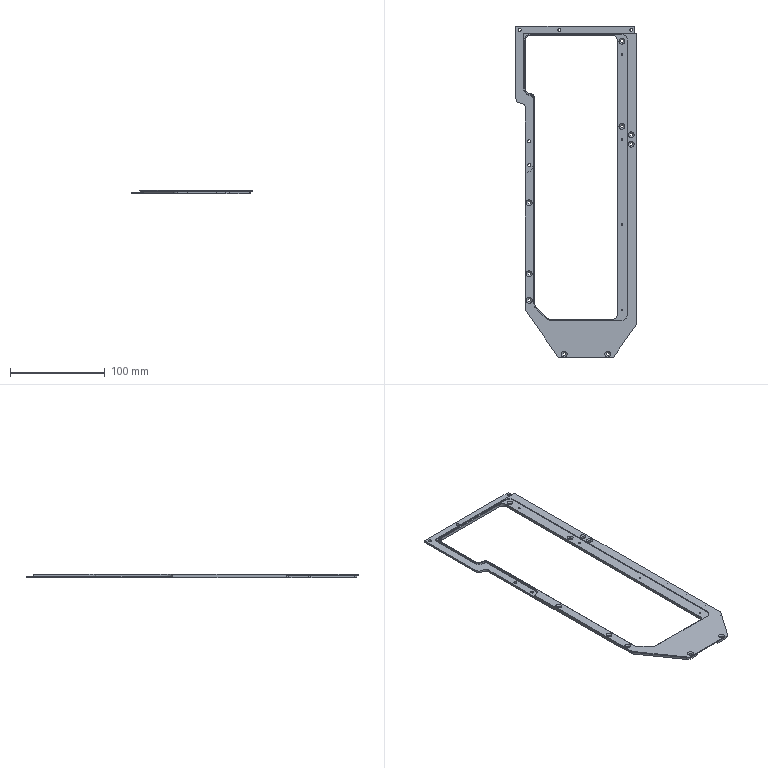NC program | NX | posted with a generic post | part box 127 x 351 x 4 mm
Whole program:
N10 G17 G21 G94 G90
(DRILLING , TOOL : CHAMFER_D8-90DEG)
N12 T01 M6
N14 G54
N16 G17 G0 G90 X-8. Y49.5 S2500 M3
N18 G43 Z20. H1
N20 G94 G81 G99 Z-2.8 F250. R3.
N22 X-83.
N24 X-111.
N26 X-168. Y12.5
N28 Y-33.5
N30 X54. Y-58.5
N32 X64.
N34 G80
N36 G0 X64. Y-58.5 Z20.
N38 M5
(PLANAR_MILL_2 , TOOL : D6-18-D6-50-3T-ROUGH)
N40 T03 M6
N42 G54
N44 G17 G0 G90 X31.2 Y59.5 S3500 M3
N46 G43 Z20. H3
N48 Z2.05
N50 G94 G1 Z-0.95 F1000.
N52 Y53.5
N54 G3 X32. Y52.7 R0.8
N56 G1 X98.935
N58 G2 X112.5 Y62.7 R14.2
N60 G1 X170.9
N62 G2 X178.2 Y55.4 R7.3
N64 G1 Y-64.6
N66 Y-70.6
N68 Z2.05
N70 G0 Z20.
N72 X27. Y59.5
N74 Z2.05
N76 G1 Z-0.95
N78 Y53.5
N80 G3 X32. Y48.5 R5.
N82 G1 X102.5
N84 G2 X112.5 Y58.5 R10.
N86 G1 X170.9
N88 G2 X174. Y55.4 R3.1
N90 G1 Y-64.6
N92 Y-70.6
N94 Z2.05
N96 G0 Z20.
N98 X31.2 Y59.5
N100 Z1.1
N102 G1 Z-1.9
N104 Y53.5
N106 G3 X32. Y52.7 R0.8
N108 G1 X98.935
N110 G2 X112.5 Y62.7 R14.2
N112 G1 X170.9
N114 G2 X178.2 Y55.4 R7.3
N116 G1 Y-64.6
N118 Y-70.6
N120 Z1.1
N122 G0 Z20.
N124 X27. Y59.5
N126 Z1.1
N128 G1 Z-1.9
N130 Y53.5
N132 G3 X32. Y48.5 R5.
N134 G1 X102.5
N136 G2 X112.5 Y58.5 R10.
N138 G1 X170.9
N140 G2 X174. Y55.4 R3.1
N142 G1 Y-64.6
N144 Y-70.6
N146 Z1.1
N148 G0 Z20.
(PLANAR_MILL_2_COPY , TOOL : D6-18-D6-50-3T-ROUGH)
N150 X90.5 Y57.5
N152 Z0.1
N154 G1 Z-1.9
N156 Y54.5
N158 G3 X92.5 Y52.5 R2.
N160 X98.5 Y58.5 R6.
N162 G2 X102.5 Y62.5 R4.
N164 G1 X175.
N166 G2 X178. Y59.5 R3.
N168 G1 Y48.5
N170 G3 X180. Y46.5 R2.
N172 G1 X183.
N174 Z0.1
N176 G0 Z20.
(PLANAR_MILL_3_COPY , TOOL : D6-18-D6-50-3T-ROUGH)
N178 X-123.5 Y-37.5
N180 Z2.1
N182 G1 Z-0.9
N184 Y-43.5
N186 Y-46.
N188 X161.5
N190 Y-43.5
N192 Y-37.5
N194 Z2.1
N196 G0 Z20.
(PLANAR_MILL_3 , TOOL : D6-18-D6-50-3T-ROUGH)
N198 X163.9 Y-48.4
N200 Z2.1
N202 G1 Z-0.9
N204 X164.
N206 Y-51.4
N208 G3 X166.9 Y-48.5 R2.9
N210 G1 Y48.5
N212 G3 X164. Y51.4 R2.9
N214 G1 X112.5
N216 G3 X109.6 Y48.5 R2.9
N218 G2 X102.5 Y41.4 R7.1
N220 G1 X-114.787
N222 G3 X-116.837 Y40.551 R2.9
N224 G1 X-128.051 Y29.337
N226 G3 X-128.9 Y27.287 R2.9
N228 G1 Y-48.5
N230 G3 X-126. Y-51.4 R2.9
N232 G1 X164.
N234 Y-48.4
N236 X163.9
N238 Z2.1
N240 G0 Z20.
N242 M5
(PLANAR_MILL_2_COPY_1 , TOOL : D6-18-D6-50-3T-FINISH)
N244 T04 M6
N246 G54
N248 G17 G0 G90 X31.1 Y59.5 S3500 M3
N250 G43 Z20. H4
N252 Z1.
N254 G94 G1 Z-2. F1000.
N256 Y53.5
N258 G3 X32. Y52.6 R0.9
N260 G1 X99.009
N262 G2 X112.5 Y62.6 R14.1
N264 G1 X170.9
N266 G2 X178.1 Y55.4 R7.2
N268 G1 Y-64.6
N270 Y-70.6
N272 Z1.
N274 G0 Z20.
N276 X26.9 Y59.5
N278 Z1.
N280 G1 Z-2.
N282 Y53.5
N284 G3 X32. Y48.4 R5.1
N286 G1 X102.5
N288 X102.565 Y48.387
N290 X102.613 Y48.435
N292 X102.6 Y48.5
N294 G2 X112.5 Y58.4 R9.9
N296 G1 X170.9
N298 G2 X173.9 Y55.4 R3.
N300 G1 Y-64.6
N302 Y-70.6
N304 Z1.
N306 G0 Z20.
(PLANAR_MILL_2_COPY_COPY , TOOL : D6-18-D6-50-3T-FINISH)
N308 X90.5 Y57.5
N310 Z0.
N312 G1 Z-2.
N314 Y54.5
N316 G3 X92.5 Y52.5 R2.
N318 X98.5 Y58.5 R6.
N320 G2 X102.5 Y62.5 R4.
N322 G1 X175.
N324 G2 X178. Y59.5 R3.
N326 G1 Y48.5
N328 G3 X180. Y46.5 R2.
N330 G1 X183.
N332 Z0.
N334 G0 Z20.
(PLANAR_MILL_3_COPY_1 , TOOL : D6-18-D6-50-3T-FINISH)
N336 X164. Y-48.5
N338 Z2.
N340 G1 Z-1.
N342 G41 Y-51.5 D40
N344 G3 X167. Y-48.5 R3.
N346 G1 Y48.5
N348 G3 X164. Y51.5 R3.
N350 G1 X112.5
N352 G3 X109.5 Y48.5 R3.
N354 G2 X102.5 Y41.5 R7.
N356 G1 X-114.787
N358 G3 X-116.908 Y40.621 R3.
N360 G1 X-128.121 Y29.408
N362 G3 X-129. Y27.287 R3.
N364 G1 Y-48.5
N366 G3 X-126. Y-51.5 R3.
N368 G1 X164.
N370 G40
N372 Y-48.5
N374 Z2.
N376 G0 Z20.
(PLANAR_MILL_3_COPY_1_COPY , TOOL : D6-18-D6-50-3T-FINISH)
N378 X163. Y-47.5
N380 Z2.
N382 G1 Z-1.
N384 X164.
N386 Y-50.5
N388 G3 X166. Y-48.5 R2.
N390 G1 Y48.5
N392 G3 X164. Y50.5 R2.
N394 G1 X112.5
N396 G3 X110.5 Y48.5 R2.
N398 G2 X102.5 Y40.5 R8.
N400 G1 X-114.787
N402 G3 X-116.201 Y39.914 R2.
N404 G1 X-127.414 Y28.701
N406 G3 X-128. Y27.287 R2.
N408 G1 Y-48.5
N410 G3 X-126. Y-50.5 R2.
N412 G1 X164.
N414 Y-47.5
N416 X163.
N418 Z2.
N420 G0 Z20.
(PLANAR_MILL_3_COPY_COPY , TOOL : D6-18-D6-50-3T-FINISH)
N422 X-123.5 Y-37.5
N424 Z2.
N426 G1 Z-1.
N428 Y-43.5
N430 Y-46.
N432 X161.5
N434 Y-43.5
N436 Y-37.5
N438 Z2.
N440 G0 Z20.
N442 M5
(DRILLING_2 , TOOL : CHAMFER_D8-90DEG)
N444 T01 M6
N446 G54
N448 G17 G0 G90 X163. Y-48.5 S2500 M3
N450 G43 Z20. H1
N452 G94 G81 G99 Z-3.8 F200. R2.
N454 X73.
N456 G80
N458 G0 X73. Y-48.5 Z20.
(DRILLING_1 , TOOL : CHAMFER_D8-90DEG)
N460 X149.
N462 G81 Z-1.8 F200. R2.
N464 X59.
N466 X-31.
N468 X-121.
N470 G80
N472 G0 X-121. Y-48.5 Z20.
N474 M5
(DRILLING_3 , TOOL : DRILL_D1.84-11-D3-40)
N476 T20 M6
N478 G54
N480 G17 G0 G90 X149. Y-48.5 S1600 M3
N482 G43 Z20. H20
N484 G94 G83 G99 Z-6. F100. Q1. R2.
N486 X59.
N488 X-31.
N490 X-121.
N492 G80
N494 G0 X-121. Y-48.5 Z20.
N496 M5
(PLANAR_MILL_5 , TOOL : CHAMFER_D3-90DEG)
N498 T08 M6
N500 G54
N502 G17 G0 G90 X173.097 Y-62.535 S3000 M3
N504 G43 Z20. H8
N506 Z1.
N508 G94 G1 Z-1. F1000.
N510 G41 X172.9 Y-62.5 D8
N512 G3 X171.9 Y-63.5 R1.
N514 G2 X170.9 Y-64.5 R1.
N516 G1 X-136.369
N518 G2 X-138.09 Y-63.957 R3.
N520 G1 X-171.721 Y-40.409
N522 G2 X-173. Y-37.952 R3.
N524 G1 Y17.098
N526 G2 X-171.721 Y19.556 R3.
N528 G1 X-122.59 Y53.957
N530 G2 X-120.869 Y54.5 R3.
N532 G1 X23.9
N534 G2 X24.9 Y53.5 R1.
N536 G3 X32. Y46.4 R7.1
N538 G1 X102.5
N540 G3 X104.6 Y48.5 R2.1
N542 G2 X112.5 Y56.4 R7.9
N544 G1 X170.9
N546 G2 X171.9 Y55.4 R1.
N548 G1 Y-63.5
N550 G3 X172.9 Y-64.5 R1.
N552 G40
N554 G1 X173.097 Y-64.465
N556 Z1.
N558 G0 Z20.
(PLANAR_MILL_5_COPY , TOOL : CHAMFER_D3-90DEG)
N560 X164.965 Y52.485
N562 Z1.2
N564 G1 Z-0.8
N566 G41 X165. Y52.682
N568 Y52.8
N570 G3 X164. Y53.8 R1.
N572 G1 X112.5
N574 G3 X107.2 Y48.5 R5.3
N576 G2 X102.5 Y43.8 R4.7
N578 G1 X-114.787
N580 G3 X-118.534 Y42.248 R5.3
N582 G1 X-129.748 Y31.034
N584 G3 X-131.3 Y27.287 R5.3
N586 G1 Y-48.5
N588 G3 X-126. Y-53.8 R5.3
N590 G1 X164.
N592 G3 X169.3 Y-48.5 R5.3
N594 G1 Y48.5
N596 G3 X164. Y53.8 R5.3
N598 X163. Y52.8 R1.
N600 G40
N602 G1 X163.035 Y52.603
N604 Z1.2
N606 G0 Z20.
(PLANAR_MILL_6 , TOOL : CHAMFER_D3-90DEG)
N608 X24.535 Y56.697
N610 Z-1.
N612 G1 Z-3.
N614 G41 X24.5 Y56.5
N616 G3 X26.5 Y54.5 R2.
N618 G1 X92.5
N620 G3 X96.5 Y58.5 R4.
N622 G2 X102.5 Y64.5 R6.
N624 G1 X179.
N626 G2 X180. Y63.5 R1.
N628 G1 Y-61.5
N630 G3 X182. Y-63.5 R2.
N632 G40
N634 G1 X182.197 Y-63.465
N636 Z-1.
N638 G0 Z20.
N640 M5
(DRILLING_3_COPY , TOOL : EXTRUDE_M2-12-D3-39)
N642 T21 M6
N644 G54
N646 G17 G0 G90 X149. Y-48.5 S300 M3
N648 G43 Z20. H21
N650 G84 G94 G99 Z-5. F120. R2.
N652 X59.
N654 X-31.
N656 X-121.
N658 G80
N660 G0 X-121. Y-48.5 Z20.
N662 M5
(PLANAR_MILL_4 , TOOL : D6-18-D6-50-3T-ROUGH)
N664 T03 M6
N666 G54
N668 G17 G0 G90 X110.726 Y49.025 S3500 M3
N670 G43 Z20. H3
N672 Z-0.5
N674 G94 G1 X110.65 Y48.835 F1500.
N676 Y48.5
N678 Y47.8 Z-0.501
N680 X110.268 Y45.935 Z-0.502
N682 X109.464 Y44.209 Z-0.503
N684 X108.284 Y42.716 Z-0.504
N686 X106.791 Y41.536 Z-0.505
N688 X105.065 Y40.732 Z-0.506
N690 X103.2 Y40.35 Z-0.507
N692 X-115.121 Z-0.621
N694 X-115.858 Y40.045
N696 X-127.545 Y28.358 Z-0.63
N698 X-127.85 Y27.621
N700 Y-38.835 Z-0.665
N702 X-127.569 Y-39.535 Z-0.666
N704 X-127.035 Y-40.069
N706 X-126.335 Y-40.35
N708 X164.335 Z-0.819
N710 X165.035 Y-40.069
N712 X165.569 Y-39.535
N714 X165.85 Y-38.835 Z-0.82
N716 Y48.835 Z-0.866
N718 X165.569 Y49.535
N720 X165.035 Y50.069
N722 X164.335 Y50.35 Z-0.867
N724 X112.165 Z-0.894
N726 X111.465 Y50.069 Z-0.895
N728 X110.931 Y49.535
N730 X110.65 Y48.835
N732 Y48.5 Z-0.896
N734 Y47.8
N736 X110.268 Y45.935 Z-0.897
N738 X109.464 Y44.209 Z-0.898
N740 X108.284 Y42.716 Z-0.899
N742 X106.791 Y41.536 Z-0.9
N744 X105.065 Y40.732 Z-0.901
N746 X103.2 Y40.35 Z-0.902
N748 X-115.121 Z-1.016
N750 X-115.858 Y40.045 Z-1.017
N752 X-127.545 Y28.358 Z-1.025
N754 X-127.85 Y27.621 Z-1.026
N756 Y-38.835 Z-1.061
N758 X-127.569 Y-39.535
N760 X-127.035 Y-40.069
N762 X-126.335 Y-40.35 Z-1.062
N764 X164.335 Z-1.214
N766 X165.035 Y-40.069
N768 X165.569 Y-39.535 Z-1.215
N770 X165.85 Y-38.835
N772 Y48.835 Z-1.261
N774 X165.569 Y49.535
N776 X165.035 Y50.069 Z-1.262
N778 X164.335 Y50.35
N780 X112.165 Z-1.289
N782 X111.465 Y50.069 Z-1.29
N784 X110.931 Y49.535
N786 X110.65 Y48.835 Z-1.291
N788 Y48.5
N790 Y47.8
N792 X110.268 Y45.935 Z-1.292
N794 X109.464 Y44.209 Z-1.293
N796 X108.284 Y42.716 Z-1.294
N798 X106.791 Y41.536 Z-1.295
N800 X105.065 Y40.732 Z-1.296
N802 X103.2 Y40.35 Z-1.297
N804 X-115.121 Z-1.411
N806 X-115.858 Y40.045 Z-1.412
N808 X-127.545 Y28.358 Z-1.421
N810 X-127.85 Y27.621
N812 Y-38.835 Z-1.456
N814 X-127.569 Y-39.535
N816 X-127.035 Y-40.069 Z-1.457
N818 X-126.335 Y-40.35
N820 X164.335 Z-1.609
N822 X165.035 Y-40.069 Z-1.61
N824 X165.569 Y-39.535
N826 X165.85 Y-38.835
N828 Y48.835 Z-1.656
N830 X165.569 Y49.535 Z-1.657
N832 X165.035 Y50.069
N834 X164.335 Y50.35
N836 X112.165 Z-1.685
N838 X111.465 Y50.069
N840 X110.931 Y49.535 Z-1.686
N842 X110.65 Y48.835
N844 Y48.5
N846 Y47.8
N848 X110.268 Y45.935 Z-1.687
N850 X109.464 Y44.209 Z-1.688
N852 X108.284 Y42.716 Z-1.689
N854 X106.791 Y41.536 Z-1.69
N856 X105.065 Y40.732 Z-1.691
N858 X103.2 Y40.35 Z-1.692
N860 X-115.121 Z-1.807
N862 X-115.858 Y40.045
N864 X-127.545 Y28.358 Z-1.816
N866 X-127.85 Y27.621
N868 Y-38.835 Z-1.851
N870 X-127.569 Y-39.535
N872 X-127.035 Y-40.069 Z-1.852
N874 X-126.335 Y-40.35
N876 X164.335 Z-2.004
N878 X165.035 Y-40.069 Z-2.005
N880 X165.569 Y-39.535
N882 X165.85 Y-38.835 Z-2.006
N884 Y48.835 Z-2.052
N886 X165.569 Y49.535
N888 X165.035 Y50.069
N890 X164.335 Y50.35 Z-2.053
N892 X112.165 Z-2.08
N894 X111.465 Y50.069
N896 X110.931 Y49.535 Z-2.081
N898 X110.65 Y48.835
N900 Y48.5
N902 Y47.8 Z-2.082
N904 X110.268 Y45.935 Z-2.083
N906 X109.464 Y44.209 Z-2.084
N908 X108.284 Y42.716 Z-2.085
N910 X106.791 Y41.536 Z-2.086
N912 X105.065 Y40.732 Z-2.087
N914 X103.2 Y40.35 Z-2.088
N916 X-115.121 Z-2.202
N918 X-115.858 Y40.045
N920 X-127.545 Y28.358 Z-2.211
N922 X-127.85 Y27.621 Z-2.212
N924 Y-38.835 Z-2.246
N926 X-127.569 Y-39.535 Z-2.247
N928 X-127.035 Y-40.069
N930 X-126.335 Y-40.35 Z-2.248
N932 X164.335 Z-2.4
N934 X165.035 Y-40.069
N936 X165.569 Y-39.535 Z-2.401
N938 X165.85 Y-38.835
N940 Y48.835 Z-2.447
N942 X165.569 Y49.535
N944 X165.035 Y50.069 Z-2.448
N946 X164.335 Y50.35
N948 X112.165 Z-2.475
N950 X111.465 Y50.069 Z-2.476
N952 X110.931 Y49.535
N954 X110.65 Y48.835
N956 Y48.5 Z-2.477
N958 Y47.8
N960 X110.268 Y45.935 Z-2.478
N962 X109.464 Y44.209 Z-2.479
N964 X108.284 Y42.716 Z-2.48
N966 X106.791 Y41.536 Z-2.481
N968 X105.065 Y40.732 Z-2.482
N970 X103.2 Y40.35 Z-2.483
N972 X-115.121 Z-2.597
N974 X-115.858 Y40.045 Z-2.598
N976 X-127.545 Y28.358 Z-2.606
N978 X-127.85 Y27.621 Z-2.607
N980 Y-38.835 Z-2.642
N982 X-127.569 Y-39.535
N984 X-127.035 Y-40.069
N986 X-126.335 Y-40.35 Z-2.643
N988 X164.335 Z-2.795
N990 X165.035 Y-40.069
N992 X165.569 Y-39.535 Z-2.796
N994 X165.85 Y-38.835
N996 Y48.835 Z-2.842
N998 X165.569 Y49.535
N1000 X165.035 Y50.069 Z-2.843
N1002 X164.335 Y50.35
N1004 X112.165 Z-2.871
N1006 X111.465 Y50.069
N1008 X110.931 Y49.535
N1010 X110.65 Y48.835 Z-2.872
N1012 Y48.5
N1014 Y47.8
N1016 X110.268 Y45.935 Z-2.873
N1018 X109.464 Y44.209 Z-2.874
N1020 X108.284 Y42.716 Z-2.875
N1022 X106.791 Y41.536 Z-2.876
N1024 X105.065 Y40.732 Z-2.877
N1026 X103.2 Y40.35 Z-2.878
N1028 X-115.121 Z-2.993
N1030 X-115.858 Y40.045
N1032 X-127.545 Y28.358 Z-3.002
N1034 X-127.85 Y27.621
N1036 Y-38.835 Z-3.037
N1038 X-127.569 Y-39.535
N1040 X-127.035 Y-40.069 Z-3.038
N1042 X-126.335 Y-40.35
N1044 X164.335 Z-3.19
N1046 X165.035 Y-40.069 Z-3.191
N1048 X165.569 Y-39.535
N1050 X165.85 Y-38.835
N1052 Y48.835 Z-3.237
N1054 X165.569 Y49.535 Z-3.238
N1056 X165.035 Y50.069
N1058 X164.335 Y50.35 Z-3.239
N1060 X112.165 Z-3.266
N1062 X111.465 Y50.069
N1064 X110.931 Y49.535 Z-3.267
N1066 X110.65 Y48.835
N1068 Y48.5
N1070 Y47.8 Z-3.268
N1072 X110.268 Y45.935 Z-3.269
N1074 X109.464 Y44.209 Z-3.27
N1076 X108.284 Y42.716 Z-3.271
N1078 X106.791 Y41.536 Z-3.272
N1080 X105.065 Y40.732 Z-3.273
N1082 X103.2 Y40.35 Z-3.274
N1084 X-115.121 Z-3.388
N1086 X-115.858 Y40.045
N1088 X-127.545 Y28.358 Z-3.397
N1090 X-127.85 Y27.621
N1092 Y-38.835 Z-3.432
N1094 X-127.569 Y-39.535 Z-3.433
N1096 X-127.035 Y-40.069
N1098 X-126.335 Y-40.35
N1100 X164.335 Z-3.586
N1102 X165.035 Y-40.069
N1104 X165.569 Y-39.535
N1106 X165.85 Y-38.835 Z-3.587
N1108 Y48.835 Z-3.633
N1110 X165.569 Y49.535
N1112 X165.035 Y50.069
N1114 X164.335 Y50.35 Z-3.634
N1116 X112.165 Z-3.661
N1118 X111.465 Y50.069 Z-3.662
N1120 X110.931 Y49.535
N1122 X110.65 Y48.835
N1124 Y48.5
N1126 Y47.8 Z-3.663
N1128 X110.268 Y45.935 Z-3.664
N1130 X109.464 Y44.209 Z-3.665
N1132 X108.284 Y42.716 Z-3.666
N1134 X106.791 Y41.536 Z-3.667
N1136 X105.065 Y40.732 Z-3.668
N1138 X103.2 Y40.35 Z-3.669
N1140 X-115.121 Z-3.783
N1142 X-115.858 Y40.045 Z-3.784
N1144 X-127.545 Y28.358 Z-3.792
N1146 X-127.85 Y27.621 Z-3.793
N1148 Y-38.835 Z-3.827
N1150 X-127.569 Y-39.535 Z-3.828
N1152 X-127.035 Y-40.069
N1154 X-126.335 Y-40.35 Z-3.829
N1156 X164.335 Z-3.981
N1158 X165.035 Y-40.069
N1160 X165.569 Y-39.535 Z-3.982
N1162 X165.85 Y-38.835
N1164 Y48.835 Z-4.028
N1166 X165.569 Y49.535
N1168 X165.035 Y50.069 Z-4.029
N1170 X164.335 Y50.35
N1172 X112.165 Z-4.056
N1174 X111.465 Y50.069 Z-4.057
N1176 X110.931 Y49.535
N1178 X110.65 Y48.835 Z-4.058
N1180 Y48.5
N1182 Y47.8
N1184 X110.268 Y45.935 Z-4.059
N1186 X109.464 Y44.209 Z-4.06
N1188 X108.284 Y42.716 Z-4.061
N1190 X106.791 Y41.536 Z-4.062
N1192 X105.065 Y40.732 Z-4.063
N1194 X103.2 Y40.35 Z-4.064
N1196 X-115.121 Z-4.178
N1198 X-115.858 Y40.045 Z-4.179
N1200 X-127.545 Y28.358 Z-4.188
N1202 X-127.85 Y27.621
N1204 Y-38.835 Z-4.223
N1206 X-127.569 Y-39.535
N1208 X-127.035 Y-40.069 Z-4.224
N1210 X-126.335 Y-40.35
N1212 X-126.
N1214 X19. Z-4.3
N1216 X164.
N1218 G3 X165.85 Y-38.5 R1.85
N1220 G1 Y48.5
N1222 G3 X164. Y50.35 R1.85
N1224 G1 X112.5
N1226 G3 X110.65 Y48.5 R1.85
N1228 G2 X102.5 Y40.35 R8.15
N1230 G1 X-114.787
N1232 G3 X-116.095 Y39.808 R1.85
N1234 G1 X-127.308 Y28.595
N1236 G3 X-127.85 Y27.287 R1.85
N1238 G1 Y-38.5
N1240 G3 X-126. Y-40.35 R1.85
N1242 G1 X19.
N1244 Z-3.8
N1246 G0 Z20.
N1248 M5
(PLANAR_MILL_4_COPY , TOOL : D6-18-D6-50-3T-FINISH)
N1250 T04 M6
N1252 G54
N1254 G17 G0 G90 X-113.822 Y39.303 S3500 M3
N1256 G43 Z20. H4
N1258 Z-2.3
N1260 G94 G1 Z-4.3 F800.
N1262 G41 X-113.787 Y39.5 D4
N1264 G3 X-114.787 Y40.5 R1.
N1266 X-116.201 Y39.914 R2.
N1268 G1 X-127.414 Y28.701
N1270 G3 X-128. Y27.287 R2.
N1272 G1 Y-38.5
N1274 G3 X-126. Y-40.5 R2.
N1276 G1 X164.
N1278 G3 X166. Y-38.5 R2.
N1280 G1 Y48.5
N1282 G3 X164. Y50.5 R2.
N1284 G1 X112.5
N1286 G3 X110.5 Y48.5 R2.
N1288 G2 X102.5 Y40.5 R8.
N1290 G1 X-114.787
N1292 G3 X-115.787 Y39.5 R1.
N1294 G40
N1296 G1 X-115.752 Y39.303
N1298 X-113.822
N1300 G41 X-113.787 Y39.5
N1302 G3 X-114.787 Y40.5 R1.
N1304 X-116.201 Y39.914 R2.
N1306 G1 X-127.414 Y28.701
N1308 G3 X-128. Y27.287 R2.
N1310 G1 Y-38.5
N1312 G3 X-126. Y-40.5 R2.
N1314 G1 X164.
N1316 G3 X166. Y-38.5 R2.
N1318 G1 Y48.5
N1320 G3 X164. Y50.5 R2.
N1322 G1 X112.5
N1324 G3 X110.5 Y48.5 R2.
N1326 G2 X102.5 Y40.5 R8.
N1328 G1 X-114.787
N1330 G3 X-115.787 Y39.5 R1.
N1332 G1 Y38.914
N1334 G40
N1336 X-115.752 Y38.717
N1338 Z-2.3
N1340 G0 Z20.
N1342 M5
(PLANAR_MILL_5_COPY_COPY , TOOL : CHAMFER_D3-90DEG)
N1344 T08 M6
N1346 G54
N1348 G17 G0 G90 X-113.787 Y41.3 S3000 M3
N1350 G43 Z20. H8
N1352 Z-0.2
N1354 G94 G1 Z-2.2 F1000.
N1356 G3 X-114.787 Y42.3 R1.
N1358 X-117.474 Y41.187 R3.8
N1360 G1 X-128.687 Y29.974
N1362 G3 X-129.8 Y27.287 R3.8
N1364 G1 Y-38.5
N1366 G3 X-126. Y-42.3 R3.8
N1368 G1 X164.
N1370 G3 X167.8 Y-38.5 R3.8
N1372 G1 Y48.5
N1374 G3 X164. Y52.3 R3.8
N1376 G1 X112.5
N1378 G3 X108.7 Y48.5 R3.8
N1380 G2 X102.5 Y42.3 R6.2
N1382 G1 X-114.787
N1384 G3 X-115.787 Y41.3 R1.
N1386 G1 Y41.115
N1388 Z-0.2
N1390 G0 Z20.
N1392 M5
N1394 M2